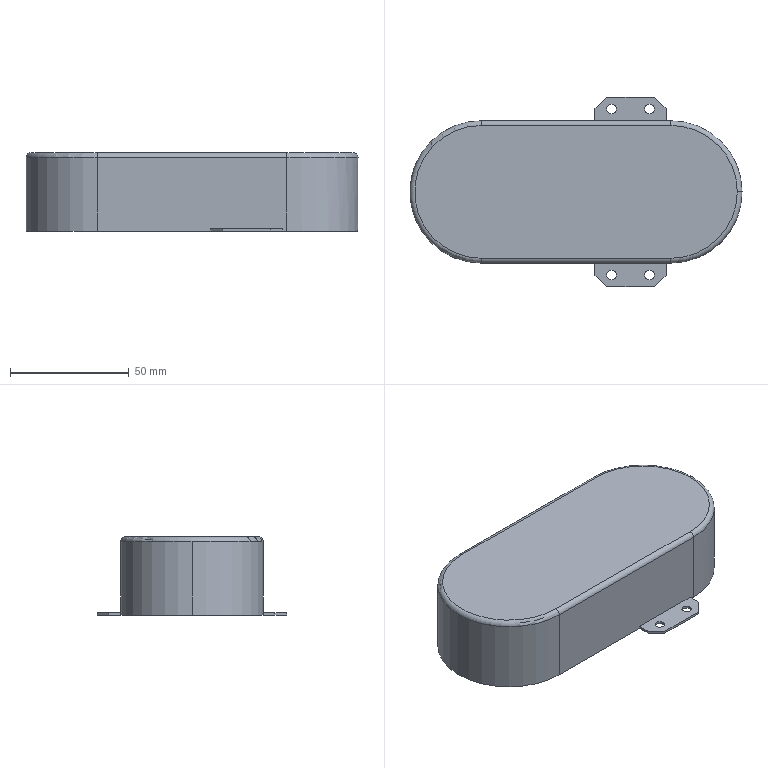Part | STEP file | 1 solid | 38 faces | box 140 x 80 x 33 mm | volume 18882 mm3 | plane 19 | cylinder 16 | torus 3 | commonest cylinder face diameters 4 x10 58 x3 60 x3